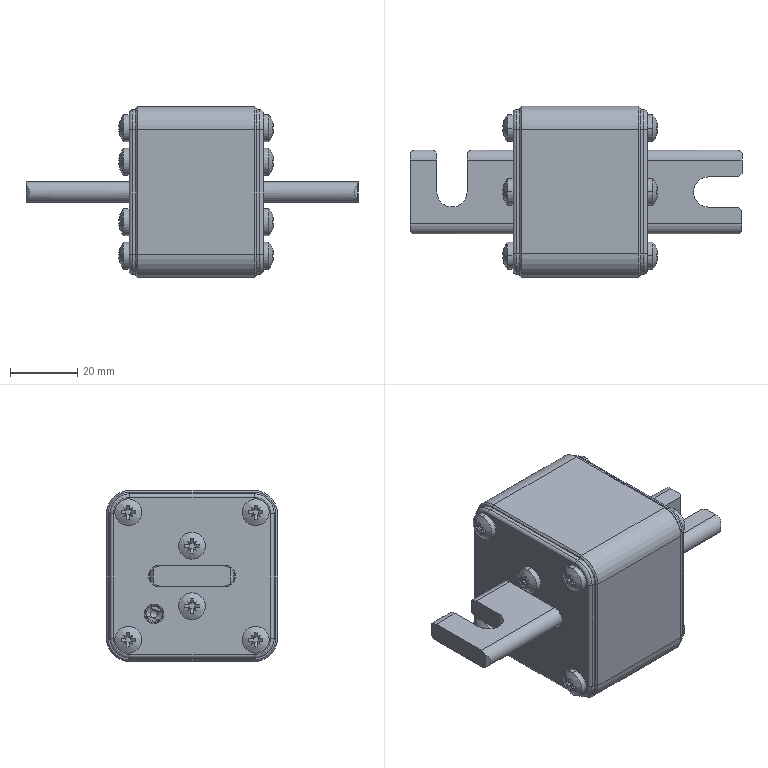Part | NX | features BREP 23 | 23 solids | 1031 faces | box 99 x 51 x 51 mm | volume 72734 mm3 | plane 607 | cylinder 343 | cone 49 | sphere 16 | torus 16 | commonest cylinder face diameters 1.6 x48 4 x48 5 x40 8 x32 3.4 x24 6 x21